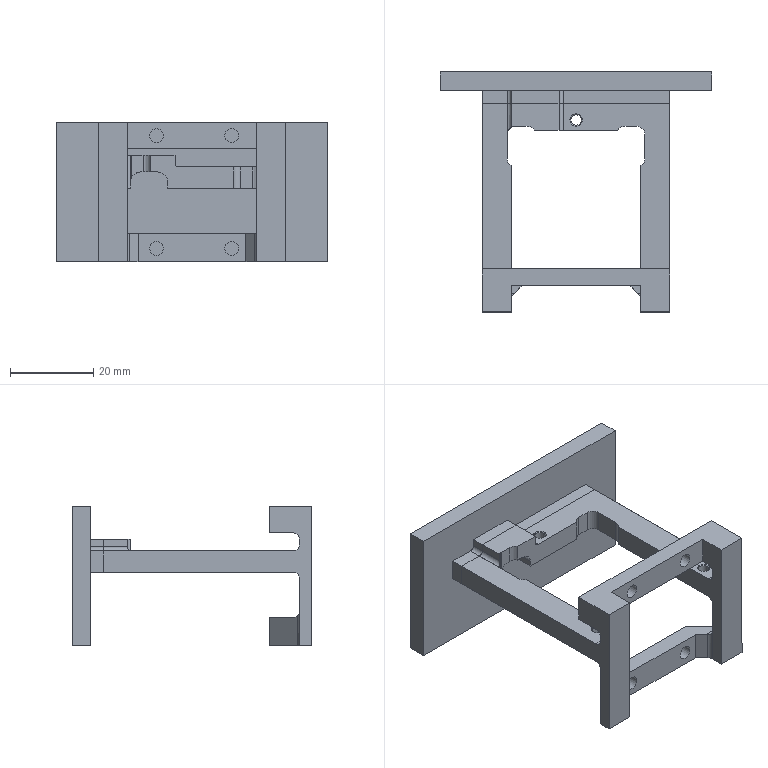NC program | NX | posted with a generic post | part box 65 x 57.5 x 33.5 mm
Lines 1 to 919 of 2388:
N10 G17 G21 G94 G90
(动态粗_1 , TOOL : D8-25-D8-60-3T-ROUGH)
N12 T02 M6
N14 G54
N16 G17 G0 G90 X42.178 Y-33.472 S6500 M3
N18 G43 Z70.5 H2
N20 Z4.1
N22 G94 G1 X42.41 Y-33.378 Z2.539 F3000.
N24 X42.642 Y-33.284 Z1.921
N26 X42.873 Y-33.19 Z1.466
N28 X43.105 Y-33.097 Z1.1
N30 X43.337 Y-33.003 Z0.793
N32 X43.568 Y-32.909 Z0.529
N34 X43.8 Y-32.815 Z0.3
N36 X44.032 Y-32.721 Z0.1
N38 X44.263 Y-32.627 Z-0.076
N40 X44.495 Y-32.533 Z-0.23
N42 X44.727 Y-32.439 Z-0.365
N44 X44.958 Y-32.345 Z-0.483
N46 X45.19 Y-32.251 Z-0.584
N48 X45.422 Y-32.157 Z-0.67
N50 X45.654 Y-32.063 Z-0.741
N52 X45.885 Y-31.969 Z-0.799
N54 X46.117 Y-31.875 Z-0.843
N56 X46.349 Y-31.781 Z-0.875
N58 X46.58 Y-31.688 Z-0.894
N60 X46.812 Y-31.594 Z-0.9
N62 X48.297 Y-30.991
N64 G3 X48.192 Y-29.472 R0.8
N66 X45.454 Y-29.095 R10.914
N68 X36.897 Y-29. R219.547
N70 G1 X21.785 Y-28.998
N72 G2 X18.525 Y-27.786 R6.157
N74 G3 X16.927 Y-26.747 R12.011
N76 G1 X16.649 Y-26.7
N78 X16.124
N80 G2 X17.086 Y-26.77 R2.738
N82 X18.92 Y-27.696 R26.256
N84 G3 X22.774 Y-28.575 R10.865
N86 X28.621 Y-28.699 R86.633
N88 G2 X44.105 Y-28.756 R832.668
N90 X48.274 Y-29.201 R21.21
N92 X48.36 Y-30.642 R0.797
N94 G1 X48.135 Y-30.724 Z-0.885
N96 X47.896 Y-30.736 Z-0.87
N98 X46.821 Y-30.47 Z-0.8
N100 X46.607 Y-30.415 F15000.
N102 X46.471 Y-30.392
N104 X46.332 Y-30.394
N106 X46.196 Y-30.419
N108 X46.067 Y-30.467
N110 X45.947 Y-30.536
N112 X45.842 Y-30.625
N114 X45.753 Y-30.732
N116 X45.684 Y-30.851
N118 X45.636 Y-30.981
N120 X45.612 Y-31.117
N122 X45.611 Y-31.255
N124 X45.634 Y-31.392
N126 X45.681 Y-31.522
N128 X45.749 Y-31.642
N130 X45.836 Y-31.749
N132 X45.941 Y-31.839
N134 X46.176 Y-32.008
N136 X46.286 Y-32.075
N138 X46.407 Y-32.123
N140 X46.533 Y-32.151
N142 X46.662 Y-32.158
N144 X46.791 Y-32.145
N146 X47.034 Y-32.056 Z-0.816 F3000.
N148 X47.237 Y-31.894 Z-0.833
N150 X47.914 Y-31.143 Z-0.89
N152 X48.592 Y-30.391 Z-0.9
N154 G3 X48.262 Y-29.108 R0.794
N156 X45.371 Y-28.431 R8.857
N158 X38.313 Y-28.206 R80.49
N160 G2 X25.11 Y-28.158 R875.286
N162 X20.987 Y-27.669 R17.181
N164 X18.292 Y-26.722 R42.74
N166 G1 X18.099 Y-26.7
N168 X16.749
N170 G2 X18.492 Y-26.727 R14.778
N172 X21.118 Y-27.362 R124.468
N174 G3 X26.862 Y-27.87 R30.838
N176 X38.939 Y-27.911 R920.696
N178 G2 X45.505 Y-28.184 R61.23
N180 X48.095 Y-28.848 R8.297
N182 X48.758 Y-29.5 R1.218
N184 X48.193 Y-30.547 R0.888
N186 G1 X46.818 Y-31.343 Z-0.8
N188 X46.683 Y-31.421 F15000.
N190 X46.561 Y-31.478
N192 X46.431 Y-31.515
N194 X46.296 Y-31.528
N196 X46.162 Y-31.519
N198 X46.03 Y-31.488
N200 X45.906 Y-31.435
N202 X45.793 Y-31.361
N204 X45.693 Y-31.27
N206 X45.611 Y-31.164
N208 X45.51 Y-31.008
N210 X45.447 Y-30.89
N212 X45.404 Y-30.762
N214 X45.383 Y-30.629
N216 X45.385 Y-30.494
N218 X45.41 Y-30.362
N220 X45.456 Y-30.236
N222 X45.523 Y-30.119
N224 X45.608 Y-30.015
N226 X45.71 Y-29.927
N228 X45.825 Y-29.857
N230 X45.95 Y-29.807
N232 X46.082 Y-29.779
N234 X46.216 Y-29.774
N236 X46.35 Y-29.791
N238 X46.479 Y-29.83
N240 X46.786 Y-29.953
N242 X47.688 Y-30.304 Z-0.861 F3000.
N244 X47.935 Y-30.322 Z-0.877
N246 X48.175 Y-30.263 Z-0.892
N248 X48.286 Y-30.206 Z-0.9
N250 X48.387 Y-30.133
N252 G3 X48.296 Y-28.853 R0.796
N254 X46.043 Y-27.935 R5.535
N256 X41.067 Y-27.469 R28.708
N258 X28.284 Y-27.382 R768.44
N260 G2 X22.711 Y-27.055 R40.844
N262 G1 X20.728 Y-26.7
N264 X18.215
N266 X21.253
N268 G3 X26.875 Y-27.047 R165.261
N270 X38.617 Y-27.125 R970.22
N272 G2 X44.936 Y-27.484 R49.98
N274 X47.823 Y-28.35 R8.48
N276 X48.769 Y-29.346 R1.949
N278 G1 X48.8 Y-29.552
N280 Y-29.396
N282 G3 X48.012 Y-28.263 R1.749
N284 X45.274 Y-27.186 R6.964
N286 X40.513 Y-26.7 R29.17
N288 G1 X21.238
N290 G3 X20.994 Y-28.262 R0.8
N292 G1 X22.525 Y-28.686 Z-0.8
N294 X23.237 Y-28.883 F15000.
N296 X23.343 Y-28.905
N298 X23.45 Y-28.912
N300 X38.3
N302 X38.417 Y-28.904
N304 X38.531 Y-28.878
N306 X38.64 Y-28.836
N308 X38.742 Y-28.779
N310 X38.835 Y-28.708
N312 X38.991 Y-28.516 Z-0.816 F3000.
N314 X39.406 Y-27.807 Z-0.869
N316 X39.822 Y-27.096 Z-0.9
N318 G2 X40.513 Y-26.7 R0.8
N320 G1 X43.1
N322 G2 X47.316 Y-27.635 R10.481
N324 X48.742 Y-28.933 R2.997
N326 G1 X48.8 Y-29.241
N328 Y-29.428
N330 Y-29.053
N332 G3 X48.007 Y-27.834 R2.013
N334 X45.508 Y-26.7 R5.553
N336 G1 X43.071
N338 X45.696
N340 G2 X48.575 Y-28.255 R4.087
N342 X48.8 Y-28.864 R1.013
N344 G1 Y-29.089
N346 Y-28.677
N348 G3 X47.949 Y-27.357 R2.135
N350 X46.708 Y-26.704 R2.791
N352 G1 X46.645 Y-26.7
N354 X45.67
N356 G2 X46.926 Y-26.72 R14.013
N358 X48.771 Y-28.255 R2.627
N360 G1 X48.8 Y-28.469
N362 Y-28.694
N364 Y-28.281
N366 G3 X47.761 Y-26.863 R2.087
N368 X47.245 Y-26.7 R0.924
N370 G1 X46.757
N372 G2 X47.561 Y-26.732 R3.77
N374 X48.788 Y-27.973 R1.854
N376 G1 X48.8 Y-28.099
N378 Y-28.286
N380 Y-27.911
N382 G3 X47.76 Y-26.711 R1.417
N384 G1 X47.647 Y-26.7
N386 X47.347
N388 G2 X48.253 Y-26.895 R1.302
N390 X48.8 Y-27.776 R1.188
N392 G1 Y-27.926
N394 Y-27.607
N396 X48.793 Y-27.497
N398 X48.785 Y-27.461
N400 G3 X47.431 Y-26.82 R0.947
N402 X48.798 Y-27.603 R-0.895
N404 G1 X48.785 Y-27.461
N406 G3 X47.705 Y-26.7 R0.935
N408 X46.922 Y-27.308 R0.808
N410 G1 X46.568 Y-28.693
N412 X46.506 Y-28.936 Z-0.894
N414 X46.445 Y-29.178 Z-0.875
N416 X46.383 Y-29.42 Z-0.843
N418 X46.321 Y-29.662 Z-0.799
N420 X46.259 Y-29.905 Z-0.741
N422 X46.197 Y-30.147 Z-0.67
N424 X46.135 Y-30.389 Z-0.584
N426 X46.073 Y-30.631 Z-0.483
N428 X46.011 Y-30.873 Z-0.365
N430 X45.95 Y-31.116 Z-0.23
N432 X45.888 Y-31.358 Z-0.076
N434 X45.826 Y-31.6 Z0.1
N436 X45.764 Y-31.842 Z0.3
N438 X45.702 Y-32.085 Z0.529
N440 X45.64 Y-32.327 Z0.793
N442 X45.578 Y-32.569 Z1.1
N444 X45.516 Y-32.811 Z1.466
N446 X45.455 Y-33.053 Z1.921
N448 X45.393 Y-33.296 Z2.539
N450 X45.331 Y-33.538 Z4.1
N452 G0 Z70.5
N454 X25.359 Y2.445
N456 Z21.75
N458 G3 X25.359 Y2.445 Z21.355 I2.665 J-2.42
N460 X25.359 Y2.445 Z20.96 I2.665 J-2.42
N462 X25.359 Y2.445 Z20.566 I2.665 J-2.42
N464 X25.359 Y2.445 Z20.171 I2.665 J-2.42
N466 X25.359 Y2.445 Z19.776 I2.665 J-2.42
N468 X25.359 Y2.445 Z19.381 I2.665 J-2.42
N470 X25.359 Y2.445 Z18.986 I2.665 J-2.42
N472 X25.359 Y2.445 Z18.591 I2.665 J-2.42
N474 X25.359 Y2.445 Z18.197 I2.665 J-2.42
N476 X25.359 Y2.445 Z17.802 I2.665 J-2.42
N478 X25.359 Y2.445 Z17.407 I2.665 J-2.42
N480 X25.359 Y2.445 Z17.012 I2.665 J-2.42
N482 X25.359 Y2.445 Z16.617 I2.665 J-2.42
N484 X25.359 Y2.445 Z16.222 I2.665 J-2.42
N486 X25.359 Y2.445 Z15.828 I2.665 J-2.42
N488 X25.359 Y2.445 Z15.433 I2.665 J-2.42
N490 X25.359 Y2.445 Z15.038 I2.665 J-2.42
N492 X25.359 Y2.445 Z14.643 I2.665 J-2.42
N494 X25.359 Y2.445 Z14.248 I2.665 J-2.42
N496 X25.359 Y2.445 Z13.854 I2.665 J-2.42
N498 X25.359 Y2.445 Z13.459 I2.665 J-2.42
N500 X25.359 Y2.445 Z13.064 I2.665 J-2.42
N502 X25.359 Y2.445 Z12.669 I2.665 J-2.42
N504 X25.359 Y2.445 Z12.274 I2.665 J-2.42
N506 X25.359 Y2.445 Z11.879 I2.665 J-2.42
N508 X25.359 Y2.445 Z11.485 I2.665 J-2.42
N510 X25.359 Y2.445 Z11.09 I2.665 J-2.42
N512 X25.359 Y2.445 Z10.695 I2.665 J-2.42
N514 X25.359 Y2.445 Z10.3 I2.665 J-2.42
N516 X25.359 Y2.445 Z9.905 I2.665 J-2.42
N518 X25.359 Y2.445 Z9.51 I2.665 J-2.42
N520 X25.359 Y2.445 Z9.116 I2.665 J-2.42
N522 X25.359 Y2.445 Z8.721 I2.665 J-2.42
N524 X25.359 Y2.445 Z8.326 I2.665 J-2.42
N526 X25.359 Y2.445 Z7.931 I2.665 J-2.42
N528 X25.359 Y2.445 Z7.536 I2.665 J-2.42
N530 X25.359 Y2.445 Z7.142 I2.665 J-2.42
N532 X25.359 Y2.445 Z6.747 I2.665 J-2.42
N534 X25.359 Y2.445 Z6.352 I2.665 J-2.42
N536 X25.359 Y2.445 Z5.957 I2.665 J-2.42
N538 X25.359 Y2.445 Z5.562 I2.665 J-2.42
N540 X25.359 Y2.445 Z5.167 I2.665 J-2.42
N542 X25.359 Y2.445 Z4.773 I2.665 J-2.42
N544 X25.359 Y2.445 Z4.378 I2.665 J-2.42
N546 X25.359 Y2.445 Z3.983 I2.665 J-2.42
N548 X25.359 Y2.445 Z3.588 I2.665 J-2.42
N550 X25.359 Y2.445 Z3.193 I2.665 J-2.42
N552 X25.359 Y2.445 Z2.798 I2.665 J-2.42
N554 X25.359 Y2.445 Z2.404 I2.665 J-2.42
N556 X25.359 Y2.445 Z2.009 I2.665 J-2.42
N558 X25.359 Y2.445 Z1.614 I2.665 J-2.42
N560 X25.359 Y2.445 Z1.219 I2.665 J-2.42
N562 X25.359 Y2.445 Z0.824 I2.665 J-2.42
N564 X25.359 Y2.445 Z0.429 I2.665 J-2.42
N566 X25.359 Y2.445 Z0.035 I2.665 J-2.42
N568 X25.359 Y2.445 Z-0.36 I2.665 J-2.42
N570 X25.359 Y2.445 Z-0.755 I2.665 J-2.42
N572 X28.025 Y-3.575 Z-0.9 R3.6
N574 X24.522 Y1.031 R-3.622
N576 X27.128 Y-3.556 R3.732
N578 X31.671 Y1.237 R3.72
N580 X26.006 Y-3.302 R-3.866
N582 X31.688 Y1.815 R3.965
N584 X25.772 Y-3.436 R-4.101
N586 X31.792 Y2.131 R4.208
N588 X25.287 Y-3.377 R-4.34
N590 X31.93 Y2.385 R4.456
N592 X24.913 Y-3.383 R-4.588
N594 X32.111 Y2.576 R4.71
N596 X24.822 Y-3.647 R-4.843
N598 X32.061 Y3.105 R4.97
N600 X24.484 Y-3.692 R-5.104
N602 X32.345 Y3.17 R5.234
N604 X24.079 Y-3.662 R-5.371
N606 X32.534 Y3.37 R5.505
N608 X23.617 Y-3.545 R-5.643
N610 X32.932 Y3.288 R5.781
N612 X23.427 Y-3.757 R-5.922
N614 X33.233 Y3.344 R6.063
N616 X23.014 Y-3.689 R-6.206
N618 X33.721 Y3.08 R6.348
N620 X22.552 Y-3.533 R-6.495
N622 X34.11 Y2.965 R6.641
N624 X22.352 Y-3.769 R-6.79
N626 X34.637 Y2.488 R6.937
N628 X21.95 Y-3.695 R-7.088
N630 X34.97 Y2.457 R7.238
N632 X21.372 Y-3.275 R-7.392
N634 X35.33 Y2.349 R7.544
N636 X20.914 Y-3.021 R-7.7
N638 X35.711 Y2.162 R7.856
N640 X20.443 Y-2.679 R-8.014
N642 X36.106 Y1.896 R8.171
N644 X19.971 Y-2.246 R-8.331
N646 X36.369 Y2.179 R8.492
N648 X19.663 Y-2.352 R-8.655
N650 X36.722 Y2.094 R8.816
N652 X19.015 Y0.198 R8.976
N654 X37.242 Y0.962 R-9.138
N656 X18.953 Y2.231 R9.3
N658 X37.135 Y-2.937 R9.459
N660 X19.666 Y4.872 R9.62
N662 X35.454 Y-6.496 R9.777
N664 X23.35 Y8.851 R9.932
N666 X27.748 Y-10.117 R10.079
N668 X31.021 Y9.896 R10.226
N670 X22.044 Y-8.521 R10.379
N672 X36.042 Y7.034 R10.536
N674 X18.733 Y-5.371 R10.699
N676 X38.594 Y3.013 R10.863
N678 X17.178 Y-2.203 R11.028
N680 X37.257 Y-6.447 R11.178
N682 X39.3 Y-1.09 R11.019
N684 G1 Y0.823
N686 G3 X29.514 Y11.301 R11.232
N688 G1 X27.039
N690 G3 X18.4 Y6.152 R11.042
N692 X25.895 Y-11.3 R11.474
N694 G1 X29.645 Y-11.301
N696 G3 X35.087 Y-9.198 R10.174
N698 X39.296 Y-3.013 R11.305
N700 G1 X39.3 Y-2.946
N702 Y-1.071
N704 Y-3.133
N706 G2 X38.272 Y-5.963 R7.114
N708 X31.121 Y-11.295 R11.351
N710 G1 X31.037 Y-11.301
N712 X29.612
N714 X31.562
N716 G3 X34.645 Y-10.187 R7.144
N718 X39.274 Y-4.663 R11.037
N720 G1 X39.3 Y-4.46
N722 Y-3.11
N724 X39.286 Y-4.738
N726 G2 X38.015 Y-7.388 R6.774
N728 X32.92 Y-11.216 R10.627
N730 X32.519 Y-11.301 R1.245
N732 G1 X31.544
N734 X32.894
N736 G3 X35.522 Y-10.265 R5.907
N738 X39.253 Y-5.923 R9.947
N740 G1 X39.3 Y-5.646
N742 Y-4.596
N744 G2 X39.28 Y-5.937 R20.151
N746 X37.966 Y-8.359 R6.106
N748 X33.934 Y-11.26 R9.088
N750 G1 X33.671 Y-11.301
N752 X32.883
N754 X34.008
N756 G3 X36.413 Y-10.277 R5.227
N758 X39.266 Y-6.914 R8.368
N760 X39.365 Y-6.398 R0.978
N762 G1 X39.3 Y-5.768
N764 G2 X39.351 Y-6.804 R3.68
N766 X37.946 Y-9.198 R5.565
N768 X34.834 Y-11.285 R7.213
N770 G1 X34.676 Y-11.301
N772 X34.001
N774 X34.976
N776 G3 X37.188 Y-10.311 R4.609
N778 X39.419 Y-7.493 R6.539
N780 X39.459 Y-6.848 R0.941
N782 G1 X39.39 Y-6.632
N784 X39.374 Y-6.483
N786 G3 X39.518 Y-7.065 R4.066
N788 G2 X38.929 Y-8.732 R3.041
N790 X35.666 Y-11.309 R6.276
N792 G1 X35.342 Y-11.337
N794 X35.001 Y-11.301
N796 X34.964
N798 X35.001
N800 X35.566 Y-11.362
N802 G3 X37.489 Y-10.642 R3.554
N804 X39.612 Y-7.935 R5.333
N806 X39.624 Y-7.362 R0.932
N808 G1 X39.486 Y-6.933
N810 G2 X39.688 Y-7.698 R2.75
N812 X38.829 Y-9.629 R3.527
N814 X36.189 Y-11.41 R4.933
N816 G1 X35.898 Y-11.398
N818 X35.56 Y-11.361
N820 G3 X36.314 Y-11.455 R7.675
N822 X38.61 Y-10.277 R3.914
N824 X39.847 Y-8.09 R3.919
N826 X39.741 Y-7.609 R0.883
N828 G1 X39.655 Y-7.458
N830 G2 X39.783 Y-8.706 R1.302
N832 X36.668 Y-11.528 R4.322
N834 X36.212 Y-11.503 R0.907
N836 G1 X35.963 Y-11.42
N838 X36.389 Y-11.562
N840 G3 X38.034 Y-11.197 R2.439
N842 X40.023 Y-8.644 R4.001
N844 X39.94 Y-7.959 R0.928
N846 G1 X39.773 Y-7.666
N848 G2 X40.084 Y-8.363 R1.711
N850 X39.313 Y-10.318 R2.958
N852 X36.949 Y-11.69 R3.648
N854 G1 X36.642 Y-11.646
N856 X36.358 Y-11.551
N858 G3 X38.189 Y-11.489 R2.004
N860 X40.242 Y-8.93 R3.645
N862 X40.087 Y-8.216 R0.892
N864 G1 X40.084 Y-8.213
N866 X39.991 Y-8.05
N868 G2 X40.279 Y-8.593 R1.938
N870 X39.662 Y-10.472 R2.595
N872 X37.266 Y-11.846 R3.311
N874 X36.749 Y-11.682 R0.925
N876 G3 X38.087 Y-11.837 R1.477
N878 X40.465 Y-9.147 R3.343
N880 X40.256 Y-8.407 R0.908
N882 G1 X40.107 Y-8.238
N884 G2 X40.496 Y-9.418 R1.175
N886 X37.724 Y-12.013 R3.262
N888 X37.117 Y-11.901 R0.971
N890 G1 X36.956 Y-11.805
N892 X37.278 Y-11.997
N894 G3 X38.917 Y-11.827 R1.996
N896 X40.693 Y-9.312 R3.126
N898 X40.475 Y-8.655 R0.896
N900 G1 X40.326 Y-8.486
N902 G2 X40.705 Y-9.785 R1.247
N904 X37.972 Y-12.2 R3.121
N906 X37.433 Y-12.089 R0.963
N908 G1 X37.271 Y-11.993
N910 X37.433 Y-12.089
N912 G3 X38.215 Y-12.3 R1.201
N914 X40.917 Y-9.534 R3.014
N916 X40.661 Y-8.864 R0.884
N918 G1 X40.535 Y-8.722
N920 G2 X40.94 Y-9.334 R1.263
N922 X40.287 Y-11.328 R2.495
N924 X38.766 Y-12.296 R2.741
N926 G1 X38.701 Y-12.3
N928 X38.214
N930 X38.926
N932 G3 X40.903 Y-10.754 R2.631
N934 X41.048 Y-9.27 R1.848
N936 X40.79 Y-8.96 R0.898
N938 G1 X40.659 Y-8.863
N940 G2 X41.201 Y-9.953 R1.075
N942 X39.401 Y-12.283 R2.696
N944 G1 X39.237 Y-12.3
N946 X38.9
N948 X39.462
N950 G3 X41.158 Y-10.894 R2.335
N952 X41.259 Y-9.411 R1.808
N954 X41.011 Y-9.124 R0.907
N956 G1 X40.83 Y-8.99
N958 G2 X41.426 Y-10.236 R1.167
N960 X39.877 Y-12.276 R2.465
N962 G1 X39.68 Y-12.3
N964 X39.455
N966 X39.868
N968 G3 X41.315 Y-11.2 R1.995
N970 X41.495 Y-9.597 R1.886
N972 X41.243 Y-9.297 R0.901
N974 G1 X41.092 Y-9.185
N976 G2 X41.66 Y-10.281 R1.095
N978 X40.277 Y-12.272 R2.236
N980 G1 X40.075 Y-12.3
N982 X39.85
N984 X40.263
N986 G3 X41.657 Y-11.086 R1.879
N988 X41.69 Y-9.7 R1.659
N990 X41.326 Y-9.358 R0.959
N992 G2 X41.883 Y-10.369 R1.013
N994 X40.622 Y-12.272 R2.03
N996 G1 X40.427 Y-12.3
N998 X40.24
N1000 X40.601
N1002 X40.676 Y-12.292
N1004 G3 X42.031 Y-10.584 R1.891
N1006 X41.636 Y-9.523 R1.103
N1008 G1 X41.526 Y-9.459
N1010 X41.389 Y-9.396
N1012 G2 X42.101 Y-10.453 R1.03
N1014 X41.688 Y-11.643 R1.591
N1016 X40.974 Y-12.226 R3.028
N1018 G1 X40.651 Y-12.295
N1020 G3 X41.402 Y-11.906 R1.059
N1022 G1 X41.688 Y-11.643
N1024 X41.748 Y-11.589
N1026 X41.834 Y-11.516
N1028 G3 X42.042 Y-9.809 R1.423
N1030 X41.73 Y-9.553 R0.898
N1032 G1 X41.593 Y-9.49
N1034 G2 X42.287 Y-10.563 R0.999
N1036 X41.928 Y-11.438 R1.084
N1038 G1 X41.813 Y-11.534
N1040 G3 X42.217 Y-9.89 R1.188
N1042 X41.905 Y-9.634 R0.898
N1044 G1 X41.768 Y-9.571
N1046 G2 X42.434 Y-10.688 R0.959
N1048 X42.007 Y-11.384 R0.902
N1050 G1 X42.192 Y-11.256
N1052 G3 X42.081 Y-9.715 R0.939
N1054 G1 X41.945 Y-9.653
N1056 X42.081 Y-9.715
N1058 X42.298 Y-9.852
N1060 G2 X42.18 Y-11.265 R0.898
N1062 G1 X42.241 Y-11.223
N1064 X42.292 Y-11.181
N1066 G3 X42.286 Y-9.843 R0.827
N1068 X41.356 Y-9.381 R6.917
N1070 G2 X39.655 Y-7.458 R4.532
N1072 X39.3 Y-5.768 R4.877
N1074 G1 Y2.36
N1076 G3 X37.786 Y6.515 R8.858
N1078 X31.309 Y11.292 R11.527
N1080 G1 X31.201 Y11.301
N1082 X29.514
N1084 X31.389
N1086 G2 X34.346 Y10.169 R7.265
N1088 X39.282 Y3.698 R11.044
N1090 G1 X39.3 Y3.532
N1092 Y2.332
N1094 Y3.982
N1096 G3 X38.283 Y6.763 R6.517
N1098 X32.855 Y11.281 R10.721
N1100 G1 X32.678 Y11.301
N1102 X31.366
N1104 X32.828
N1106 G2 X35.062 Y10.377 R5.598
N1108 X39.17 Y5.395 R10.379
N1110 X39.3 Y4.863 R1.502
N1112 G1 Y3.963
N1114 Y5.201
N1116 G3 X38.341 Y7.643 R5.453
N1118 X34.1 Y11.263 R9.6
N1120 G1 X33.853 Y11.301
N1122 X32.803
N1124 X34.003
N1126 G2 X36.074 Y10.334 R4.951
N1128 X39.236 Y6.283 R8.814
N1130 X39.3 Y5.947 R0.975
N1132 G1 Y5.197
N1134 Y6.247
N1136 G3 X38.324 Y8.554 R4.868
N1138 X35.08 Y11.27 R7.732
N1140 G1 X34.851 Y11.301
N1142 X33.989
N1144 X35.001
N1146 G2 X36.918 Y10.331 R4.282
N1148 X39.28 Y7.087 R7.001
N1150 G1 X39.3 Y6.91
N1152 Y6.235
N1154 Y7.172
N1156 G3 X38.387 Y9.262 R4.259
N1158 X35.821 Y11.329 R6.026
N1160 G1 X35.505 Y11.355
N1162 X35.007 Y11.301
N1164 X34.969
N1166 G2 X35.815 Y11.358 R4.757
N1168 X37.837 Y10.159 R4.312
N1170 X39.288 Y7.905 R5.354
N1172 G1 X39.3 Y7.77
N1174 Y7.17
N1176 Y8.032
N1178 G3 X38.221 Y10.158 R3.935
N1180 X36.35 Y11.439 R4.252
N1182 X35.944 Y11.412 R0.896
N1184 G1 X35.9 Y11.397
N1186 X35.602 Y11.365
N1188 G3 X36.198 Y11.474 R4.316
N1190 G2 X37.716 Y10.827 R2.733
N1192 X39.285 Y8.679 R4.512
N1194 G1 X39.3 Y8.521
N1196 Y7.996
N1198 Y8.783
N1200 G3 X38.098 Y10.835 R3.433
N1202 X36.644 Y11.591 R2.743
N1204 G1 X36.353 Y11.548
N1206 X35.997 Y11.43
N1208 G2 X36.826 Y11.604 R1.738
N1210 X38.916 Y10.111 R3.34
N1212 X39.3 Y9.185 R1.922
N1214 G1 Y8.772
N1216 Y9.41
N1218 G3 X37.914 Y11.399 R2.893
N1220 X36.868 Y11.711 R1.544
N1222 G1 X36.751 Y11.682
N1224 X36.431 Y11.575
N1226 G2 X37.229 Y11.74 R1.625
N1228 X39.285 Y9.889 R2.778
N1230 G1 X39.3 Y9.733
N1232 Y9.395
N1234 Y9.958
N1236 G3 X37.319 Y11.876 R2.373
N1238 X36.752 Y11.682 R0.975
N1240 G2 X37.962 Y11.77 R1.124
N1242 X39.3 Y10.303 R2.273
N1244 G1 X39.308 Y10.109
N1246 X39.3 Y10.011
N1248 Y9.936
N1250 Y10.011
N1252 X39.322 Y10.296
N1254 G3 X38.203 Y11.842 R1.935
N1256 X37.133 Y11.909 R1.095
N1258 G1 X36.94 Y11.794
N1260 G2 X38.312 Y11.867 R1.177
N1262 X39.331 Y10.635 R1.87
N1264 G1 X39.335 Y10.47
N1266 X39.321 Y10.283
N1268 X39.349 Y10.645
N1270 G3 X38.313 Y12.035 R1.677
N1272 X37.376 Y12.054 R0.956
N1274 G1 X37.183 Y11.939
N1276 G2 X38.541 Y11.992 R1.128
N1278 X39.368 Y10.871 R1.518
N1280 G1 X39.349 Y10.645
N1282 X39.386 Y10.803
N1284 G3 X38.78 Y11.996 R1.339
N1286 X37.541 Y12.14 R1.058
N1288 X37.477 Y10.715 R0.88
N1290 X38.217 Y10.18 R3.546
N1292 X39.343 Y11.459 R0.925
N1294 X38.36 Y12.297 R1.264
N1296 G1 X38.308 Y12.3
N1298 G3 X37.439 Y12.092 R1.281
N1300 G2 X38.804 Y12.18 R1.42
N1302 X39.434 Y11.009 R1.165
N1304 G1 X39.408 Y10.899
N1306 X39.468 Y11.155
N1308 G3 X38.568 Y12.3 R1.012
N1310 G1 X38.381
N1312 X38.633
N1314 X38.745 Y12.287
N1316 G2 X39.493 Y11.298 R0.931
N1318 G1 X39.478 Y11.199
N1320 X39.461 Y11.126
N1322 X39.478 Y11.199
N1324 X39.493 Y11.298
N1326 G3 X38.717 Y12.29 R0.838
N1328 X37.751 Y12.249 R3.036
N1330 X36.752 Y11.682 R17.201
N1332 G2 X35.007 Y11.301 R4.863
N1334 G1 X25.576 Y11.3
N1336 G3 X21.523 Y9.819 R8.726
N1338 X24.37 Y-11.288 R11.827
N1340 G1 X24.507 Y-11.3
N1342 X25.932
N1344 X24.357
N1346 G2 X21.762 Y-10.31 R6.647
N1348 X22.243 Y10.493 R12.006
N1350 X24.381 Y11.298 R8.275
N1352 G1 X24.433 Y11.3
N1354 X25.595
N1356 X23.983
N1358 G3 X21.119 Y10.219 R6.543
N1360 X15.788 Y-2.072 R12.199
N1362 X22.217 Y-10.97 R12.181
N1364 X23.156 Y-11.3 R2.583
N1366 G1 X24.393
N1368 X22.876 Y-11.285
N1370 G2 X20.326 Y-10.031 R6.584
N1372 X20.317 Y9.933 R12.555
N1374 X23.035 Y11.295 R7.886
N1376 G1 X23.119 Y11.3
N1378 X24.019
N1380 X22.782
N1382 G3 X20.384 Y10.367 R5.406
N1384 X15.548 Y3.665 R12.061
N1386 X20.031 Y-10.272 R12.926
N1388 X21.879 Y-11.288 R6.045
N1390 G1 X22.012 Y-11.3
N1392 X23.025
N1394 X21.741 Y-11.284
N1396 G2 X19.395 Y-10.022 R5.974
N1398 X14.884 Y1.543 R13.003
N1400 X19.764 Y10.198 R12.568
N1402 X21.934 Y11.293 R6.472
N1404 G1 X22.03 Y11.3
N1406 X22.818
N1408 X21.73
N1410 G3 X19.437 Y10.337 R4.933
N1412 X15.212 Y4.595 R11.98
N1414 X14.5 Y1.549 R13.348
N1416 G1 Y-1.076
N1418 G3 X19.412 Y-10.494 R12.72
N1420 X20.867 Y-11.288 R4.718
N1422 G1 X21.001 Y-11.3
N1424 X21.863
N1426 G2 X20.728 Y-11.282 R33.429
N1428 X18.547 Y-10.039 R5.481
N1430 X14.5 Y-2.843 R12.719
N1432 G1 Y-1.043
N1434 Y-3.518
N1436 G3 X15.634 Y-6.998 R8.656
N1438 X19.187 Y-10.938 R10.605
N1440 X20.077 Y-11.3 R1.912
N1442 G1 X20.902
N1444 G2 X19.804 Y-11.281 R24.078
N1446 X17.728 Y-10.045 R5.105
N1448 X14.504 Y-4.724 R10.845
N1450 G1 X14.5 Y-4.656
N1452 Y-3.493
N1454 Y-5.106
N1456 G3 X15.587 Y-8.022 R6.855
N1458 X18.678 Y-11.136 R8.643
N1460 X19.206 Y-11.3 R1.043
N1462 G1 X19.994
N1464 G2 X18.929 Y-11.279 R10.892
N1466 X16.899 Y-9.997 R4.855
N1468 X14.507 Y-6.082 R8.676
N1470 G1 X14.5 Y-5.985
N1472 Y-5.085
N1474 Y-6.36
N1476 G3 X15.606 Y-8.999 R5.751
N1478 X18.116 Y-11.252 R6.599
N1480 G1 X18.395 Y-11.3
N1482 X19.107
N1484 G2 X18.115 Y-11.277 R7.987
N1486 X16.103 Y-9.91 R4.562
N1488 X14.507 Y-7.175 R6.539
N1490 G1 X14.5 Y-7.08
N1492 Y-6.33
N1494 Y-7.38
N1496 G3 X15.54 Y-9.708 R4.644
N1498 X17.399 Y-11.26 R5.107
N1500 G1 X17.652 Y-11.3
N1502 X18.289
N1504 G2 X17.342 Y-11.27 R4.915
N1506 X15.389 Y-9.784 R4.231
N1508 X14.506 Y-8.087 R4.499
N1510 G1 X14.5 Y-8.
N1512 Y-7.363
N1514 Y-8.263
N1516 G3 X15.734 Y-10.56 R3.892
N1518 X16.842 Y-11.286 R2.599
N1520 G1 X16.997 Y-11.3
N1522 X17.559
N1524 G2 X16.681 Y-11.269 R4.222
N1526 X14.721 Y-9.442 R3.634
N1528 X14.5 Y-8.765 R1.452
N1530 G1 Y-8.24
N1532 Y-9.027
N1534 G3 X16.171 Y-11.259 R3.054
N1536 G1 X16.435 Y-11.3
N1538 X16.885
N1540 G2 X16.008 Y-11.229 R2.325
N1542 X14.506 Y-9.466 R2.628
N1544 G1 X14.5 Y-9.38
N1546 Y-9.005
N1548 Y-9.605
N1550 G3 X15.731 Y-11.262 R2.165
N1552 G1 X15.977 Y-11.3
N1554 X16.352
N1556 G2 X15.508 Y-11.201 R1.735
N1558 X14.505 Y-9.937 R1.873
N1560 G1 X14.5 Y-9.855
N1562 Y-9.592
N1564 Y-10.061
N1566 G3 X15.454 Y-11.277 R1.448
N1568 G1 X15.634 Y-11.3
N1570 X15.897
N1572 G2 X14.5 Y-10.22 R1.219
N1574 G1 Y-10.033
N1576 Y-10.393
N1578 X14.506 Y-10.486
N1580 G3 X15.348 Y-11.296 R0.97
N1582 G1 X15.407 Y-11.3
N1584 X15.595
N1586 X15.407
N1588 X15.348 Y-11.296
N1590 G2 X14.505 Y-10.465 R0.881
N1592 X15.119 Y-9.601 R0.9
N1594 G1 X16.403 Y-8.889 Z-0.808
N1596 X16.493 Y-8.808 Z-0.8
N1598 X16.571 Y-8.714 F15000.
N1600 X16.634 Y-8.608
N1602 X16.68 Y-8.494
N1604 X16.708 Y-8.375
N1606 X16.717 Y-8.252
N1608 X16.713 Y-0.663
N1610 X16.704 Y-0.546
N1612 X16.678 Y-0.432
N1614 X16.636 Y-0.323
N1616 X16.579 Y-0.221
N1618 X16.507 Y-0.128
N1620 X16.317 Y0.027 Z-0.815 F3000.
N1622 X15.607 Y0.443 Z-0.869
N1624 X14.896 Y0.859 Z-0.9
N1626 G2 X14.5 Y1.549 R0.8
N1628 G1 Y2.187
N1630 G2 X15.806 Y6.47 R10.308
N1632 X19.742 Y10.772 R11.064
N1634 X21.062 Y11.3 R3.371
N1636 G1 X21.737
N1638 X20.762
N1640 G3 X18.592 Y10.337 R4.676
N1642 X14.506 Y4.261 R11.618
N1644 G1 X14.5 Y4.169
N1646 Y2.182
N1648 Y4.357
N1650 G2 X15.547 Y7.206 R7.329
N1652 X19.089 Y10.891 R10.033
N1654 X20.168 Y11.3 R2.765
N1656 G1 X20.768
N1658 X19.905
N1660 G3 X17.888 Y10.414 R4.213
N1662 X14.516 Y5.817 R9.935
N1664 G1 X14.5 Y5.658
N1666 Y4.346
N1668 G2 X14.535 Y6.061 R12.295
N1670 X16.206 Y9.119 R7.566
N1672 X19.059 Y11.256 R7.061
N1674 G1 X19.329 Y11.3
N1676 X19.929
N1678 X19.066
N1680 G3 X17.049 Y10.364 R4.116
N1682 X14.518 Y6.999 R7.773
N1684 G1 X14.5 Y6.831
N1686 Y5.781
N1688 G2 X14.518 Y7.11 R36.099
N1690 X15.978 Y9.639 R5.777
N1692 X18.372 Y11.284 R5.679
N1694 G1 X18.533 Y11.3
N1696 X19.095
N1698 X18.27
N1700 G3 X16.271 Y10.316 R3.92
N1702 X14.527 Y7.996 R6.063
N1704 G1 X14.5 Y7.79
N1706 Y6.965
N1708 G2 X14.523 Y8.085 R9.373
N1710 X16.187 Y10.471 R4.875
N1712 X17.708 Y11.295 R3.523
N1714 G1 X17.789 Y11.3
N1716 X18.277
N1718 X17.527
N1720 G3 X15.562 Y10.249 R3.61
N1722 X14.521 Y8.763 R3.863
N1724 G1 X14.5 Y8.583
N1726 Y7.908
N1728 G2 X14.523 Y8.862 R8.095
N1730 X16.938 Y11.283 R3.876
N1732 G1 X17.101 Y11.3
N1734 X17.551
N1736 X16.876
N1738 G3 X14.925 Y10.103 R3.083
N1740 X14.5 Y9.219 R1.527
N1742 G1 Y8.694
N1744 G2 X14.532 Y9.53 R3.92
N1746 X16.404 Y11.292 R2.813
N1748 G1 X16.511 Y11.3
N1750 X16.886
N1752 X16.286
N1754 G3 X14.534 Y9.953 R2.336
N1756 G1 X14.5 Y9.716
N1758 Y9.304
N1760 G2 X14.545 Y10.064 R2.487
N1762 X15.949 Y11.295 R1.999
N1764 G1 X16.033 Y11.3
N1766 X16.296
N1768 X15.846
N1770 G3 X14.525 Y10.284 R1.576
N1772 G1 X14.5 Y10.098
N1774 Y9.798
N1776 G2 X14.626 Y10.597 R1.371
N1778 X15.651 Y11.3 R1.351
N1780 G1 X15.876
N1782 G3 X14.585 Y10.707 R1.29
N1784 X14.5 Y10.369 R0.911
N1786 G1 Y10.144
N1788 Y10.369
N1790 G2 X14.559 Y10.705 R0.884
N1792 X16.179 Y10.8 R0.886
N1794 X14.514 Y10.291 R-0.876
N1796 X14.559 Y10.705 R0.845
N1798 X15.52 Y11.3 R0.9
N1800 X16.296 Y10.717 R0.808
N1802 G1 X16.705 Y9.307
N1804 X16.774 Y9.067 Z-0.894
N1806 X16.844 Y8.826 Z-0.875
N1808 X16.914 Y8.586 Z-0.843
N1810 X16.983 Y8.346 Z-0.799
N1812 X17.053 Y8.106 Z-0.741
N1814 X17.123 Y7.866 Z-0.67
N1816 X17.192 Y7.626 Z-0.584
N1818 X17.262 Y7.386 Z-0.483
N1820 X17.331 Y7.146 Z-0.365
N1822 X17.401 Y6.906 Z-0.23
N1824 X17.471 Y6.665 Z-0.076
N1826 X17.54 Y6.425 Z0.1
N1828 X17.61 Y6.185 Z0.3
N1830 X17.679 Y5.945 Z0.529
N1832 X17.749 Y5.705 Z0.793
N1834 X17.819 Y5.465 Z1.1
N1836 X17.888 Y5.225 Z1.466